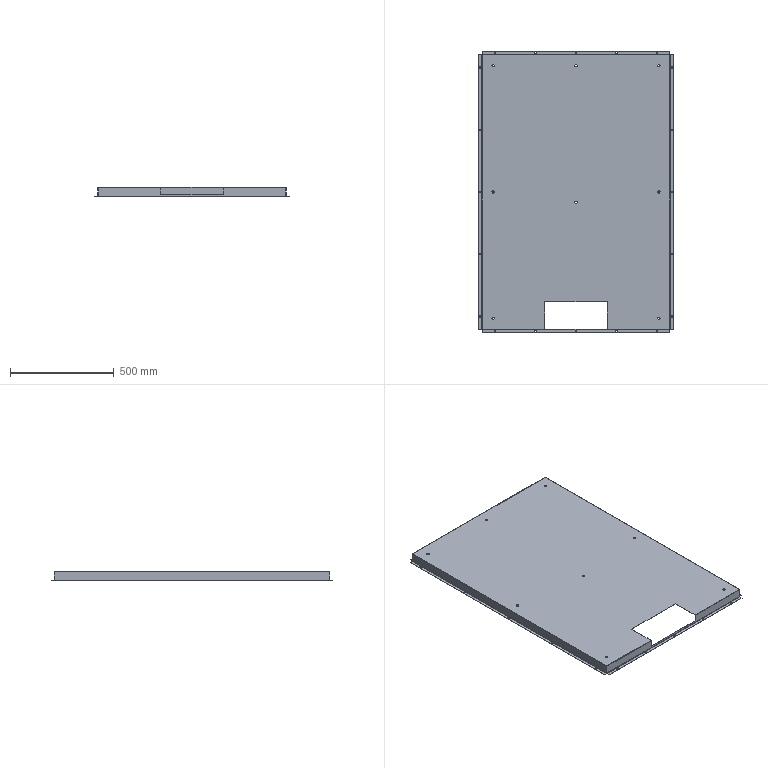Part | SolidWorks | features ICE 4, EdgeFlange 2, Cut 1, FlatPattern 1, SMBaseFlange 1, SheetMetal 1 | 1 solid | 186 faces | box 940 x 1360 x 44 mm | volume 1413374 mm3 | plane 94 | cylinder 84 | spline 8 | commonest cylinder face diameters 7 x50 11 x16 1 x9 3 x9